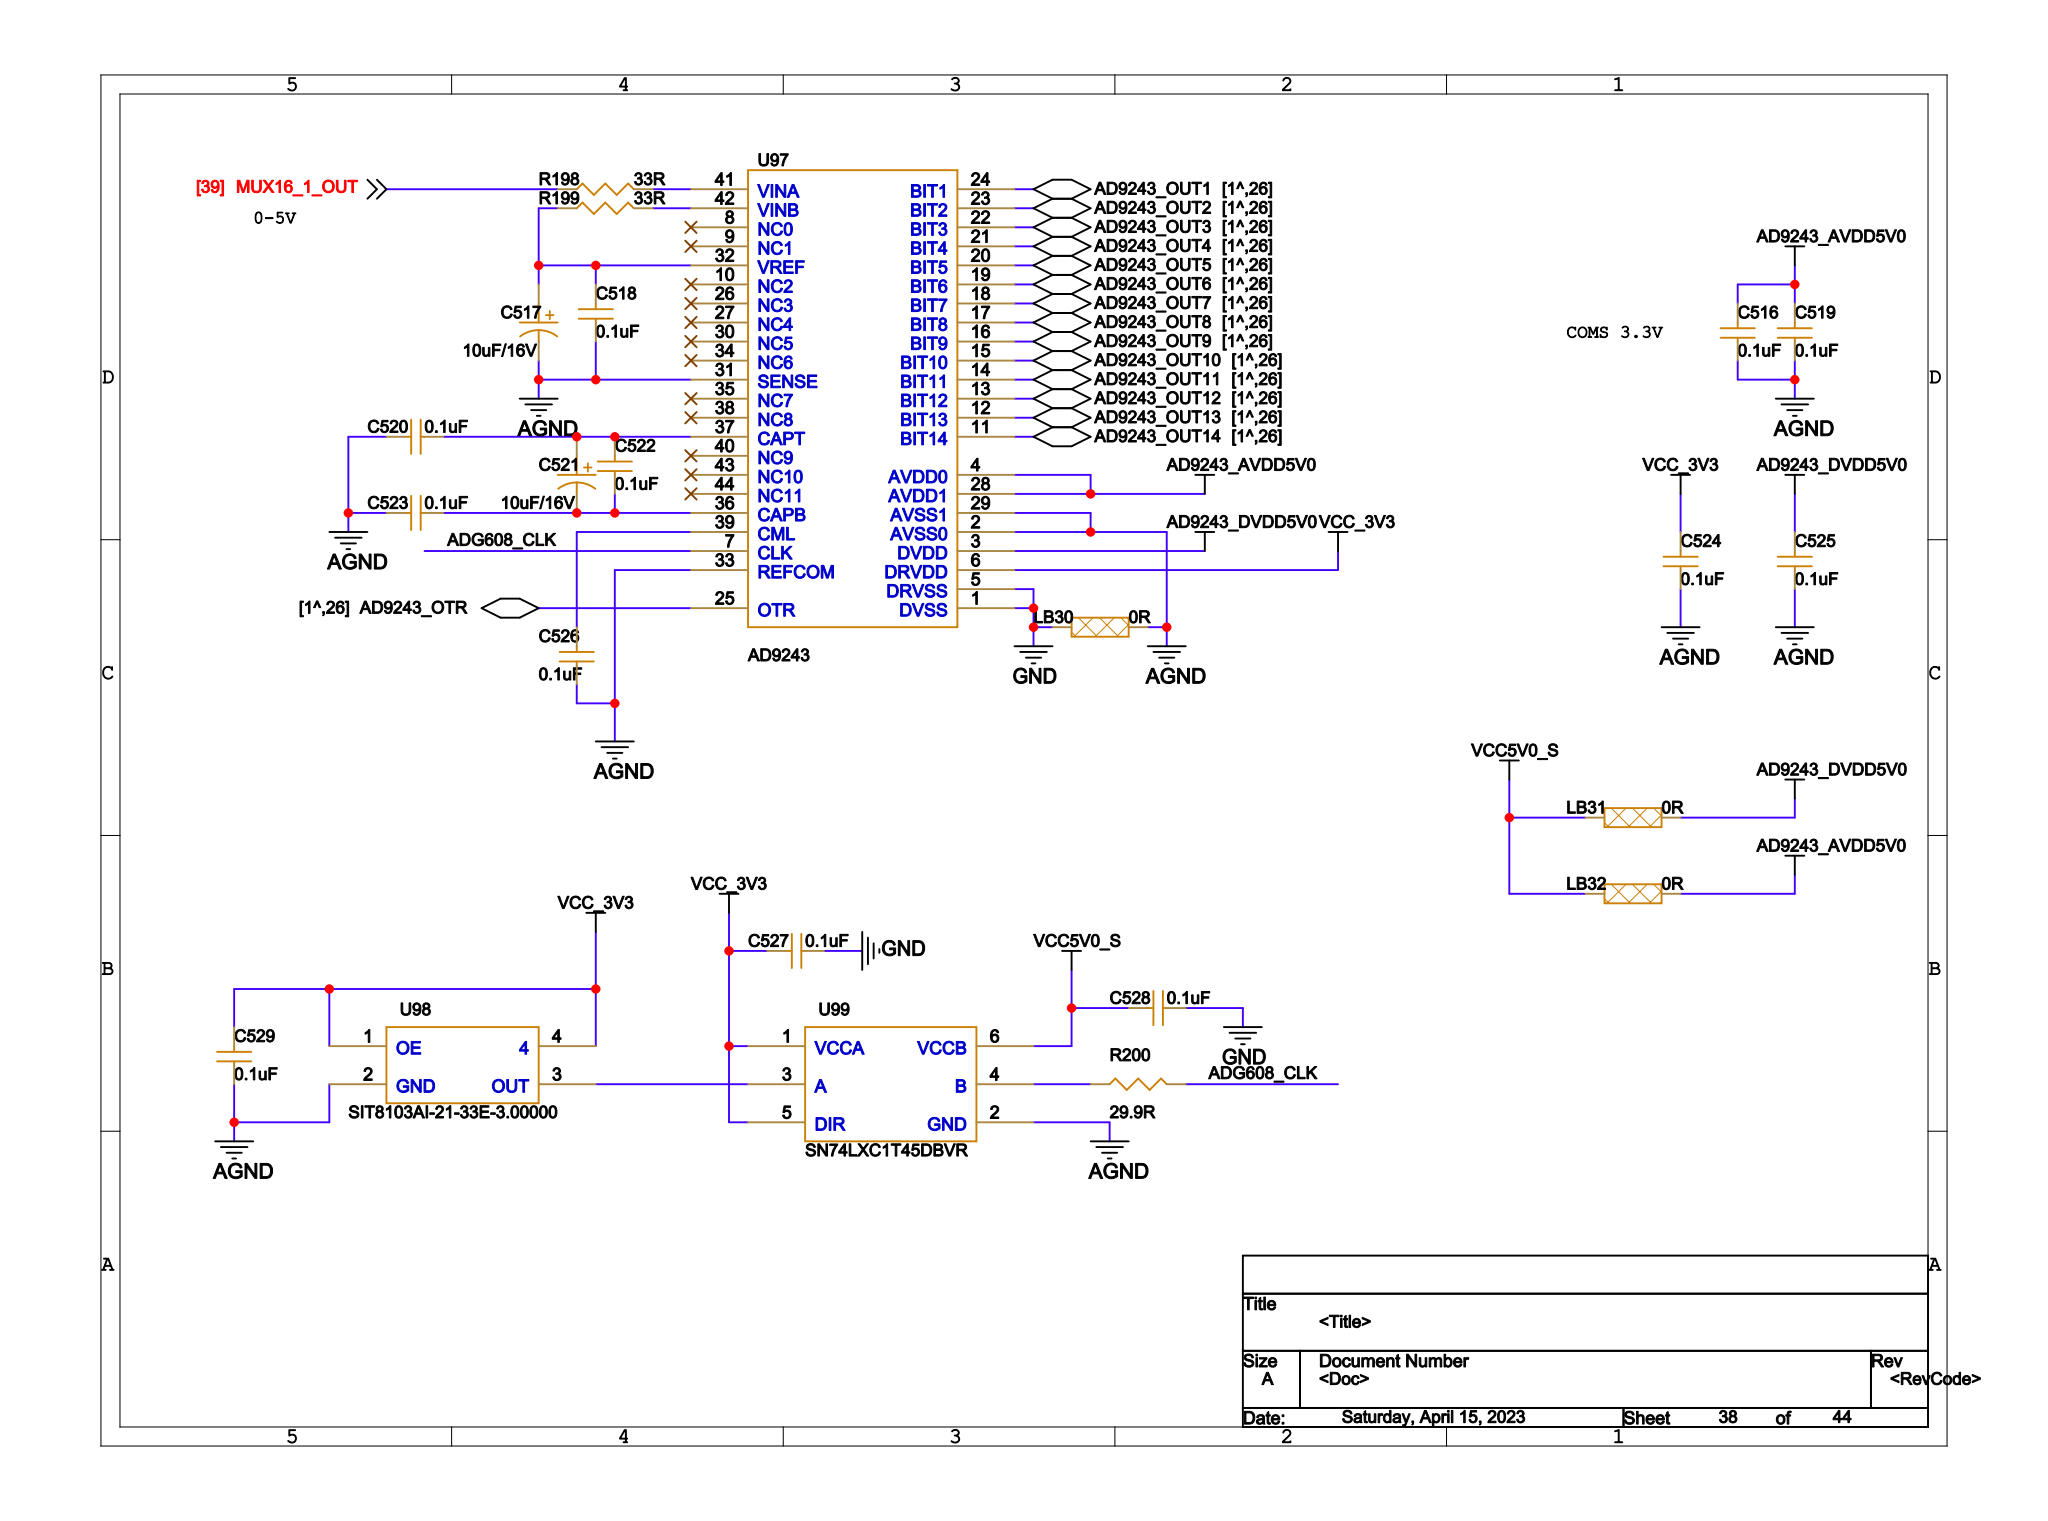Circuit board | Cadence Allegro | 1034 parts | 912 nets | one sheet of the schematic
Parts on this sheet (reference | value | footprint):
C516 | 0.1uF | C0402
C517 | 10uF/16V | C0402
C518 | 0.1uF | C0402
C519 | 0.1uF | C0402
C520 | 0.1uF | C0402
C521 | 10uF/16V | C0402
C522 | 0.1uF | C0402
C523 | 0.1uF | C0402
C524 | 0.1uF | C0402
C525 | 0.1uF | C0402
C526 | 0.1uF | C0402
C527 | 0.1uF | C0402
C528 | 0.1uF | C0402
C529 | 0.1uF | C0402
LB30 | 0R | LB0805
LB31 | 0R | LB0805
LB32 | 0R | LB0805
R198 | 33R | R0402
R199 | 33R | R0402
R200 | 29.9R | R0402
U97 | AD9243 | AD9243_MQFP
U98 | SIT8103AI-21-33E-3 | SIT_3MM2X2MM5
U99 | SN74LXC1T45DBVR | SN74LXC_SOT23
Nets of these parts (net: part-pin ...):
GND: C527-1 C528-1 LB30-1 U97-1 U97-5
VCC_3V3: C524-2 C527-2 C529-2 U98-1 U98-4 U99-1 U99-5 U97-6
AGND: C516-1 C517-2 C518-1 C519-1 C520-2 C523-2 C524-1 C525-1 C526-1 C529-1 LB30-2 U98-2 U99-2 U97-2 U97-29 U97-31 U97-33
VCC5V0_S: C528-2 LB31-1 LB32-1 U99-6
MUX16_1_OUT: R198-1
N14070505: R198-2 U97-41
N14066488: C517-1 C518-2 R199-1 U97-32
N14070501: R199-2 U97-42
N14070757: U98-3 U99-3
AD9243_AVDD5V0: C516-2 C519-2 LB32-2 U97-4 U97-28
N14069058: C520-1 C521-1 C522-2 U97-37
N14069062: C521-2 C522-1 C523-1 U97-36
AD9243_DVDD5V0: C525-2 LB31-2 U97-3
N14068890: C526-2 U97-39
N14071135: R200-1 U99-4
ADG608_CLK: R200-2 U97-7